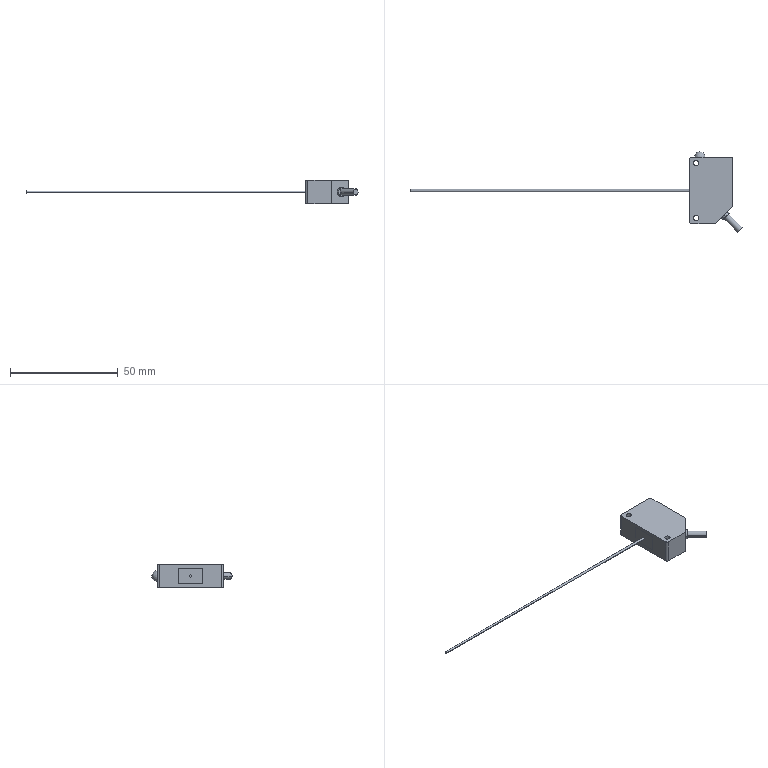Part | STEP file | ES201-R10MN (Huayifeng) | 1 solid | 26 faces | box 154.334 x 37.365 x 10.8 mm | volume 6448 mm3 | cylinder 13 | plane 11 | sphere 2 | commonest cylinder face diameters 2.5 x4 2 x3 1 x2 2.91 x2 4.315 x2
STEP:
#1=CARTESIAN_POINT('',(-140.,0.5,0.));
#2=VERTEX_POINT('',#1);
#3=CARTESIAN_POINT('',(-140.,-0.5,0.));
#4=VERTEX_POINT('',#3);
#5=CARTESIAN_POINT('',(-140.,0.,0.));
#6=DIRECTION('',(1.,0.,0.));
#7=DIRECTION('',(0.,-1.,0.));
#8=AXIS2_PLACEMENT_3D('',#5,#6,#7);
#9=CIRCLE('',#8,0.5);
#10=EDGE_CURVE('',#2,#4,#9,.T.);
#11=ORIENTED_EDGE('',*,*,#10,.T.);
#12=CARTESIAN_POINT('',(-10.,-0.5,0.));
#13=VERTEX_POINT('',#12);
#14=CARTESIAN_POINT('',(-140.,-0.5,0.));
#15=DIRECTION('',(1.,0.,0.));
#16=VECTOR('',#15,1000.);
#17=LINE('',#14,#16);
#18=EDGE_CURVE('',#4,#13,#17,.T.);
#19=ORIENTED_EDGE('',*,*,#18,.T.);
#20=CARTESIAN_POINT('',(-10.,0.5,0.));
#21=VERTEX_POINT('',#20);
#22=CARTESIAN_POINT('',(-10.,0.,0.));
#23=DIRECTION('',(1.,0.,0.));
#24=DIRECTION('',(0.,1.,0.));
#25=AXIS2_PLACEMENT_3D('',#22,#23,#24);
#26=CIRCLE('',#25,0.5);
#27=EDGE_CURVE('',#21,#13,#26,.T.);
#28=ORIENTED_EDGE('',*,*,#27,.F.);
#29=CARTESIAN_POINT('',(-140.,0.5,0.));
#30=DIRECTION('',(1.,0.,0.));
#31=VECTOR('',#30,1000.);
#32=LINE('',#29,#31);
#33=EDGE_CURVE('',#2,#21,#32,.T.);
#34=ORIENTED_EDGE('',*,*,#33,.F.);
#35=EDGE_LOOP('',(#11,#19,#28,#34));
#36=FACE_OUTER_BOUND('',#35,.T.);
#37=CARTESIAN_POINT('',(-140.,0.,0.));
#38=DIRECTION('',(1.,0.,0.));
#39=DIRECTION('',(0.,1.,0.));
#40=AXIS2_PLACEMENT_3D('',#37,#38,#39);
#41=CYLINDRICAL_SURFACE('',#40,0.5);
#42=ADVANCED_FACE('',(#36),#41,.T.);
#43=CARTESIAN_POINT('',(12.277,-19.365,0.));
#44=VERTEX_POINT('',#43);
#45=CARTESIAN_POINT('',(14.334,-17.308,0.));
#46=VERTEX_POINT('',#45);
#47=CARTESIAN_POINT('',(13.306,-18.336,0.));
#48=DIRECTION('',(-0.7071,0.7071,0.));
#49=DIRECTION('',(0.7071,0.7071,0.));
#50=AXIS2_PLACEMENT_3D('',#47,#48,#49);
#51=CIRCLE('',#50,1.455);
#52=EDGE_CURVE('',#44,#46,#51,.T.);
#53=ORIENTED_EDGE('',*,*,#52,.T.);
#54=CARTESIAN_POINT('',(7.97,-10.944,0.));
#55=VERTEX_POINT('',#54);
#56=CARTESIAN_POINT('',(14.334,-17.308,0.));
#57=DIRECTION('',(-0.7071,0.7071,0.));
#58=VECTOR('',#57,1000.);
#59=LINE('',#56,#58);
#60=EDGE_CURVE('',#46,#55,#59,.T.);
#61=ORIENTED_EDGE('',*,*,#60,.T.);
#62=CARTESIAN_POINT('',(5.913,-13.001,0.));
#63=VERTEX_POINT('',#62);
#64=CARTESIAN_POINT('',(6.942,-11.972,0.));
#65=DIRECTION('',(-0.7071,0.7071,0.));
#66=DIRECTION('',(0.7071,0.7071,0.));
#67=AXIS2_PLACEMENT_3D('',#64,#65,#66);
#68=CIRCLE('',#67,1.455);
#69=EDGE_CURVE('',#63,#55,#68,.T.);
#70=ORIENTED_EDGE('',*,*,#69,.F.);
#71=CARTESIAN_POINT('',(12.277,-19.365,0.));
#72=DIRECTION('',(-0.7071,0.7071,0.));
#73=VECTOR('',#72,1000.);
#74=LINE('',#71,#73);
#75=EDGE_CURVE('',#44,#63,#74,.T.);
#76=ORIENTED_EDGE('',*,*,#75,.F.);
#77=EDGE_LOOP('',(#53,#61,#70,#76));
#78=FACE_OUTER_BOUND('',#77,.T.);
#79=CARTESIAN_POINT('',(13.306,-18.336,0.));
#80=DIRECTION('',(-0.7071,0.7071,0.));
#81=DIRECTION('',(-0.7071,-0.7071,0.));
#82=AXIS2_PLACEMENT_3D('',#79,#80,#81);
#83=CYLINDRICAL_SURFACE('',#82,1.455);
#84=ADVANCED_FACE('',(#78),#83,.T.);
#85=CARTESIAN_POINT('',(5.416,-13.498,0.));
#86=VERTEX_POINT('',#85);
#87=CARTESIAN_POINT('',(8.467,-10.447,0.));
#88=VERTEX_POINT('',#87);
#89=CARTESIAN_POINT('',(6.942,-11.972,0.));
#90=DIRECTION('',(-0.7071,0.7071,0.));
#91=DIRECTION('',(0.7071,0.7071,0.));
#92=AXIS2_PLACEMENT_3D('',#89,#90,#91);
#93=CIRCLE('',#92,2.158);
#94=EDGE_CURVE('',#86,#88,#93,.T.);
#95=ORIENTED_EDGE('',*,*,#94,.T.);
#96=CARTESIAN_POINT('',(7.76,-9.74,0.));
#97=VERTEX_POINT('',#96);
#98=CARTESIAN_POINT('',(8.467,-10.447,0.));
#99=DIRECTION('',(-0.7071,0.7071,0.));
#100=VECTOR('',#99,1000.);
#101=LINE('',#98,#100);
#102=EDGE_CURVE('',#88,#97,#101,.T.);
#103=ORIENTED_EDGE('',*,*,#102,.T.);
#104=CARTESIAN_POINT('',(4.709,-12.791,0.));
#105=VERTEX_POINT('',#104);
#106=CARTESIAN_POINT('',(6.235,-11.265,0.));
#107=DIRECTION('',(-0.7071,0.7071,0.));
#108=DIRECTION('',(0.7071,0.7071,0.));
#109=AXIS2_PLACEMENT_3D('',#106,#107,#108);
#110=CIRCLE('',#109,2.158);
#111=EDGE_CURVE('',#105,#97,#110,.T.);
#112=ORIENTED_EDGE('',*,*,#111,.F.);
#113=CARTESIAN_POINT('',(5.416,-13.498,0.));
#114=DIRECTION('',(-0.7071,0.7071,0.));
#115=VECTOR('',#114,1000.);
#116=LINE('',#113,#115);
#117=EDGE_CURVE('',#86,#105,#116,.T.);
#118=ORIENTED_EDGE('',*,*,#117,.F.);
#119=EDGE_LOOP('',(#95,#103,#112,#118));
#120=FACE_OUTER_BOUND('',#119,.T.);
#121=CARTESIAN_POINT('',(6.942,-11.972,0.));
#122=DIRECTION('',(-0.7071,0.7071,0.));
#123=DIRECTION('',(-0.7071,-0.7071,0.));
#124=AXIS2_PLACEMENT_3D('',#121,#122,#123);
#125=CYLINDRICAL_SURFACE('',#124,2.158);
#126=ADVANCED_FACE('',(#120),#125,.T.);
#127=CARTESIAN_POINT('',(-5.75,-12.7,5.4));
#128=VERTEX_POINT('',#127);
#129=CARTESIAN_POINT('',(-8.25,-12.7,5.4));
#130=VERTEX_POINT('',#129);
#131=CARTESIAN_POINT('',(-7.,-12.7,5.4));
#132=DIRECTION('',(0.,0.,1.));
#133=DIRECTION('',(1.,0.,0.));
#134=AXIS2_PLACEMENT_3D('',#131,#132,#133);
#135=CIRCLE('',#134,1.25);
#136=EDGE_CURVE('',#128,#130,#135,.T.);
#137=ORIENTED_EDGE('',*,*,#136,.T.);
#138=CARTESIAN_POINT('',(-8.25,-12.7,-5.4));
#139=VERTEX_POINT('',#138);
#140=CARTESIAN_POINT('',(-8.25,-12.7,-5.4));
#141=DIRECTION('',(0.,0.,-1.));
#142=VECTOR('',#141,1000.);
#143=LINE('',#140,#142);
#144=EDGE_CURVE('',#130,#139,#143,.T.);
#145=ORIENTED_EDGE('',*,*,#144,.T.);
#146=CARTESIAN_POINT('',(-5.75,-12.7,-5.4));
#147=VERTEX_POINT('',#146);
#148=CARTESIAN_POINT('',(-7.,-12.7,-5.4));
#149=DIRECTION('',(0.,0.,1.));
#150=DIRECTION('',(1.,0.,0.));
#151=AXIS2_PLACEMENT_3D('',#148,#149,#150);
#152=CIRCLE('',#151,1.25);
#153=EDGE_CURVE('',#147,#139,#152,.T.);
#154=ORIENTED_EDGE('',*,*,#153,.F.);
#155=CARTESIAN_POINT('',(-5.75,-12.7,-5.4));
#156=DIRECTION('',(0.,0.,-1.));
#157=VECTOR('',#156,1000.);
#158=LINE('',#155,#157);
#159=EDGE_CURVE('',#128,#147,#158,.T.);
#160=ORIENTED_EDGE('',*,*,#159,.F.);
#161=EDGE_LOOP('',(#137,#145,#154,#160));
#162=FACE_OUTER_BOUND('',#161,.T.);
#163=CARTESIAN_POINT('',(-7.,-12.7,-5.4));
#164=DIRECTION('',(0.,0.,-1.));
#165=DIRECTION('',(1.,0.,0.));
#166=AXIS2_PLACEMENT_3D('',#163,#164,#165);
#167=CYLINDRICAL_SURFACE('',#166,1.25);
#168=ADVANCED_FACE('',(#162),#167,.F.);
#169=CARTESIAN_POINT('',(-7.176,13.938,0.));
#170=VERTEX_POINT('',#169);
#171=CARTESIAN_POINT('',(-5.806,13.069,-0.001365));
#172=VERTEX_POINT('',#171);
#173=CARTESIAN_POINT('',(-7.176,13.938,0.));
#174=CARTESIAN_POINT('',(-7.176,13.938,0.1523));
#175=CARTESIAN_POINT('',(-7.16,13.94,0.3021));
#176=CARTESIAN_POINT('',(-7.096,13.947,0.5968));
#177=CARTESIAN_POINT('',(-7.047,13.951,0.7424));
#178=CARTESIAN_POINT('',(-6.91,13.949,1.012));
#179=CARTESIAN_POINT('',(-6.821,13.943,1.139));
#180=CARTESIAN_POINT('',(-6.652,13.902,1.289));
#181=CARTESIAN_POINT('',(-6.592,13.884,1.331));
#182=CARTESIAN_POINT('',(-6.461,13.83,1.392));
#183=CARTESIAN_POINT('',(-6.393,13.795,1.408));
#184=CARTESIAN_POINT('',(-6.265,13.714,1.408));
#185=CARTESIAN_POINT('',(-6.205,13.667,1.391));
#186=CARTESIAN_POINT('',(-6.102,13.572,1.33));
#187=CARTESIAN_POINT('',(-6.059,13.525,1.287));
#188=CARTESIAN_POINT('',(-5.952,13.391,1.137));
#189=CARTESIAN_POINT('',(-5.908,13.313,1.011));
#190=CARTESIAN_POINT('',(-5.848,13.19,0.739));
#191=CARTESIAN_POINT('',(-5.831,13.145,0.5964));
#192=CARTESIAN_POINT('',(-5.81,13.084,0.3011));
#193=CARTESIAN_POINT('',(-5.806,13.069,0.1493));
#194=CARTESIAN_POINT('',(-5.806,13.069,-0.001365));
#195=B_SPLINE_CURVE_WITH_KNOTS('',3,(#173,#174,#175,#176,#177,#178,#179,#180,#181,#182,#183,#184,#185,#186,#187,#188,#189,#190,#191,#192,#193,#194),.UNSPECIFIED.,.F.,.F.,(4,2,2,2,2,2,2,2,2,2,4),(0.,0.0004516,0.0009031,0.001355,0.00158,0.001806,0.002032,0.002258,0.002709,0.003161,0.003613),.UNSPECIFIED.);
#196=EDGE_CURVE('',#170,#172,#195,.T.);
#197=ORIENTED_EDGE('',*,*,#196,.T.);
#198=CARTESIAN_POINT('',(-5.806,13.069,-0.001365));
#199=CARTESIAN_POINT('',(-5.806,13.069,-0.152));
#200=CARTESIAN_POINT('',(-5.81,13.084,-0.3044));
#201=CARTESIAN_POINT('',(-5.832,13.145,-0.5986));
#202=CARTESIAN_POINT('',(-5.848,13.191,-0.7422));
#203=CARTESIAN_POINT('',(-5.894,13.284,-0.9455));
#204=CARTESIAN_POINT('',(-5.913,13.318,-1.01));
#205=CARTESIAN_POINT('',(-5.96,13.395,-1.132));
#206=CARTESIAN_POINT('',(-5.989,13.437,-1.19));
#207=CARTESIAN_POINT('',(-6.06,13.526,-1.289));
#208=CARTESIAN_POINT('',(-6.104,13.574,-1.332));
#209=CARTESIAN_POINT('',(-6.207,13.669,-1.391));
#210=CARTESIAN_POINT('',(-6.267,13.715,-1.408));
#211=CARTESIAN_POINT('',(-6.395,13.797,-1.408));
#212=CARTESIAN_POINT('',(-6.463,13.831,-1.391));
#213=CARTESIAN_POINT('',(-6.593,13.884,-1.33));
#214=CARTESIAN_POINT('',(-6.654,13.903,-1.288));
#215=CARTESIAN_POINT('',(-6.822,13.943,-1.137));
#216=CARTESIAN_POINT('',(-6.911,13.949,-1.011));
#217=CARTESIAN_POINT('',(-7.047,13.951,-0.7418));
#218=CARTESIAN_POINT('',(-7.096,13.947,-0.5968));
#219=CARTESIAN_POINT('',(-7.16,13.94,-0.3018));
#220=CARTESIAN_POINT('',(-7.176,13.938,-0.1523));
#221=CARTESIAN_POINT('',(-7.176,13.938,0.));
#222=B_SPLINE_CURVE_WITH_KNOTS('',3,(#198,#199,#200,#201,#202,#203,#204,#205,#206,#207,#208,#209,#210,#211,#212,#213,#214,#215,#216,#217,#218,#219,#220,#221),.UNSPECIFIED.,.F.,.F.,(4,2,2,2,2,2,2,2,2,2,2,4),(0.003613,0.004064,0.004516,0.004741,0.004967,0.005193,0.005419,0.005645,0.00587,0.006322,0.006773,0.007225),.UNSPECIFIED.);
#223=EDGE_CURVE('',#172,#170,#222,.T.);
#224=ORIENTED_EDGE('',*,*,#223,.T.);
#225=EDGE_LOOP('',(#197,#224));
#226=FACE_BOUND('',#225,.T.);
#227=CARTESIAN_POINT('',(-5.75,12.7,5.4));
#228=VERTEX_POINT('',#227);
#229=CARTESIAN_POINT('',(-8.25,12.7,5.4));
#230=VERTEX_POINT('',#229);
#231=CARTESIAN_POINT('',(-7.,12.7,5.4));
#232=DIRECTION('',(0.,0.,1.));
#233=DIRECTION('',(1.,0.,0.));
#234=AXIS2_PLACEMENT_3D('',#231,#232,#233);
#235=CIRCLE('',#234,1.25);
#236=EDGE_CURVE('',#228,#230,#235,.T.);
#237=ORIENTED_EDGE('',*,*,#236,.T.);
#238=CARTESIAN_POINT('',(-8.25,12.7,-5.4));
#239=VERTEX_POINT('',#238);
#240=CARTESIAN_POINT('',(-8.25,12.7,-5.4));
#241=DIRECTION('',(0.,0.,-1.));
#242=VECTOR('',#241,1000.);
#243=LINE('',#240,#242);
#244=EDGE_CURVE('',#230,#239,#243,.T.);
#245=ORIENTED_EDGE('',*,*,#244,.T.);
#246=CARTESIAN_POINT('',(-5.75,12.7,-5.4));
#247=VERTEX_POINT('',#246);
#248=CARTESIAN_POINT('',(-7.,12.7,-5.4));
#249=DIRECTION('',(0.,0.,1.));
#250=DIRECTION('',(1.,0.,0.));
#251=AXIS2_PLACEMENT_3D('',#248,#249,#250);
#252=CIRCLE('',#251,1.25);
#253=EDGE_CURVE('',#247,#239,#252,.T.);
#254=ORIENTED_EDGE('',*,*,#253,.F.);
#255=CARTESIAN_POINT('',(-5.75,12.7,-5.4));
#256=DIRECTION('',(0.,0.,-1.));
#257=VECTOR('',#256,1000.);
#258=LINE('',#255,#257);
#259=EDGE_CURVE('',#228,#247,#258,.T.);
#260=ORIENTED_EDGE('',*,*,#259,.F.);
#261=EDGE_LOOP('',(#237,#245,#254,#260));
#262=FACE_OUTER_BOUND('',#261,.T.);
#263=CARTESIAN_POINT('',(-7.,12.7,-5.4));
#264=DIRECTION('',(0.,0.,-1.));
#265=DIRECTION('',(1.,0.,0.));
#266=AXIS2_PLACEMENT_3D('',#263,#264,#265);
#267=CYLINDRICAL_SURFACE('',#266,1.25);
#268=ADVANCED_FACE('',(#226,#262),#267,.F.);
#269=CARTESIAN_POINT('',(-10.,5.6,-3.7));
#270=VERTEX_POINT('',#269);
#271=CARTESIAN_POINT('',(-10.,5.6,3.7));
#272=VERTEX_POINT('',#271);
#273=CARTESIAN_POINT('',(-10.,5.6,-5.4));
#274=DIRECTION('',(0.,0.,1.));
#275=VECTOR('',#274,1000.);
#276=LINE('',#273,#275);
#277=EDGE_CURVE('',#270,#272,#276,.T.);
#278=ORIENTED_EDGE('',*,*,#277,.F.);
#279=CARTESIAN_POINT('',(-10.,-5.6,-3.7));
#280=VERTEX_POINT('',#279);
#281=CARTESIAN_POINT('',(-10.,15.5,-3.7));
#282=DIRECTION('',(0.,1.,0.));
#283=VECTOR('',#282,1000.);
#284=LINE('',#281,#283);
#285=EDGE_CURVE('',#280,#270,#284,.T.);
#286=ORIENTED_EDGE('',*,*,#285,.F.);
#287=CARTESIAN_POINT('',(-10.,-5.6,3.7));
#288=VERTEX_POINT('',#287);
#289=CARTESIAN_POINT('',(-10.,-5.6,-5.4));
#290=DIRECTION('',(0.,0.,-1.));
#291=VECTOR('',#290,1000.);
#292=LINE('',#289,#291);
#293=EDGE_CURVE('',#288,#280,#292,.T.);
#294=ORIENTED_EDGE('',*,*,#293,.F.);
#295=CARTESIAN_POINT('',(-10.,15.5,3.7));
#296=DIRECTION('',(0.,-1.,0.));
#297=VECTOR('',#296,1000.);
#298=LINE('',#295,#297);
#299=EDGE_CURVE('',#272,#288,#298,.T.);
#300=ORIENTED_EDGE('',*,*,#299,.F.);
#301=EDGE_LOOP('',(#278,#286,#294,#300));
#302=FACE_OUTER_BOUND('',#301,.T.);
#303=ORIENTED_EDGE('',*,*,#27,.T.);
#304=CARTESIAN_POINT('',(-10.,0.,0.));
#305=DIRECTION('',(1.,0.,0.));
#306=DIRECTION('',(0.,1.,0.));
#307=AXIS2_PLACEMENT_3D('',#304,#305,#306);
#308=CIRCLE('',#307,0.5);
#309=EDGE_CURVE('',#13,#21,#308,.T.);
#310=ORIENTED_EDGE('',*,*,#309,.T.);
#311=EDGE_LOOP('',(#303,#310));
#312=FACE_BOUND('',#311,.T.);
#313=CARTESIAN_POINT('',(-10.,15.5,-5.4));
#314=DIRECTION('',(1.,0.,0.));
#315=DIRECTION('',(0.,1.,0.));
#316=AXIS2_PLACEMENT_3D('',#313,#314,#315);
#317=PLANE('',#316);
#318=ADVANCED_FACE('',(#302,#312),#317,.F.);
#319=CARTESIAN_POINT('',(-10.,14.5,5.4));
#320=VERTEX_POINT('',#319);
#321=CARTESIAN_POINT('',(-10.,-14.5,5.4));
#322=VERTEX_POINT('',#321);
#323=CARTESIAN_POINT('',(-10.,15.5,5.4));
#324=DIRECTION('',(0.,-1.,0.));
#325=VECTOR('',#324,1000.);
#326=LINE('',#323,#325);
#327=EDGE_CURVE('',#320,#322,#326,.T.);
#328=ORIENTED_EDGE('',*,*,#327,.F.);
#329=CARTESIAN_POINT('',(-10.,14.5,-5.4));
#330=VERTEX_POINT('',#329);
#331=CARTESIAN_POINT('',(-10.,14.5,-5.4));
#332=DIRECTION('',(0.,0.,1.));
#333=VECTOR('',#332,1000.);
#334=LINE('',#331,#333);
#335=EDGE_CURVE('',#330,#320,#334,.T.);
#336=ORIENTED_EDGE('',*,*,#335,.F.);
#337=CARTESIAN_POINT('',(-10.,-14.5,-5.4));
#338=VERTEX_POINT('',#337);
#339=CARTESIAN_POINT('',(-10.,15.5,-5.4));
#340=DIRECTION('',(0.,-1.,0.));
#341=VECTOR('',#340,1000.);
#342=LINE('',#339,#341);
#343=EDGE_CURVE('',#330,#338,#342,.T.);
#344=ORIENTED_EDGE('',*,*,#343,.T.);
#345=CARTESIAN_POINT('',(-10.,-14.5,-5.4));
#346=DIRECTION('',(0.,0.,-1.));
#347=VECTOR('',#346,1000.);
#348=LINE('',#345,#347);
#349=EDGE_CURVE('',#322,#338,#348,.T.);
#350=ORIENTED_EDGE('',*,*,#349,.F.);
#351=EDGE_LOOP('',(#328,#336,#344,#350));
#352=FACE_OUTER_BOUND('',#351,.T.);
#353=ORIENTED_EDGE('',*,*,#299,.T.);
#354=ORIENTED_EDGE('',*,*,#293,.T.);
#355=ORIENTED_EDGE('',*,*,#285,.T.);
#356=ORIENTED_EDGE('',*,*,#277,.T.);
#357=EDGE_LOOP('',(#353,#354,#355,#356));
#358=FACE_BOUND('',#357,.T.);
#359=CARTESIAN_POINT('',(-10.,15.5,-5.4));
#360=DIRECTION('',(1.,0.,0.));
#361=DIRECTION('',(0.,1.,0.));
#362=AXIS2_PLACEMENT_3D('',#359,#360,#361);
#363=PLANE('',#362);
#364=ADVANCED_FACE('',(#352,#358),#363,.F.);
#365=ORIENTED_EDGE('',*,*,#94,.F.);
#366=CARTESIAN_POINT('',(6.942,-11.972,0.));
#367=DIRECTION('',(-0.7071,0.7071,0.));
#368=DIRECTION('',(0.7071,0.7071,0.));
#369=AXIS2_PLACEMENT_3D('',#366,#367,#368);
#370=CIRCLE('',#369,2.158);
#371=EDGE_CURVE('',#88,#86,#370,.T.);
#372=ORIENTED_EDGE('',*,*,#371,.F.);
#373=EDGE_LOOP('',(#365,#372));
#374=FACE_OUTER_BOUND('',#373,.T.);
#375=ORIENTED_EDGE('',*,*,#69,.T.);
#376=CARTESIAN_POINT('',(6.942,-11.972,0.));
#377=DIRECTION('',(-0.7071,0.7071,0.));
#378=DIRECTION('',(0.7071,0.7071,0.));
#379=AXIS2_PLACEMENT_3D('',#376,#377,#378);
#380=CIRCLE('',#379,1.455);
#381=EDGE_CURVE('',#55,#63,#380,.T.);
#382=ORIENTED_EDGE('',*,*,#381,.T.);
#383=EDGE_LOOP('',(#375,#382));
#384=FACE_BOUND('',#383,.T.);
#385=CARTESIAN_POINT('',(6.942,-11.972,0.));
#386=DIRECTION('',(0.7071,-0.7071,0.));
#387=DIRECTION('',(0.7071,0.7071,0.));
#388=AXIS2_PLACEMENT_3D('',#385,#386,#387);
#389=PLANE('',#388);
#390=ADVANCED_FACE('',(#374,#384),#389,.T.);
#391=CARTESIAN_POINT('',(2.,-15.5,-5.4));
#392=VERTEX_POINT('',#391);
#393=CARTESIAN_POINT('',(10.,-7.5,-5.4));
#394=VERTEX_POINT('',#393);
#395=CARTESIAN_POINT('',(6.,-11.5,-5.4));
#396=DIRECTION('',(0.7071,0.7071,0.));
#397=VECTOR('',#396,1000.);
#398=LINE('',#395,#397);
#399=EDGE_CURVE('',#392,#394,#398,.T.);
#400=ORIENTED_EDGE('',*,*,#399,.T.);
#401=CARTESIAN_POINT('',(10.,-7.5,5.4));
#402=VERTEX_POINT('',#401);
#403=CARTESIAN_POINT('',(10.,-7.5,-5.4));
#404=DIRECTION('',(0.,0.,1.));
#405=VECTOR('',#404,1000.);
#406=LINE('',#403,#405);
#407=EDGE_CURVE('',#394,#402,#406,.T.);
#408=ORIENTED_EDGE('',*,*,#407,.T.);
#409=CARTESIAN_POINT('',(2.,-15.5,5.4));
#410=VERTEX_POINT('',#409);
#411=CARTESIAN_POINT('',(10.,-7.5,5.4));
#412=DIRECTION('',(-0.7071,-0.7071,0.));
#413=VECTOR('',#412,1000.);
#414=LINE('',#411,#413);
#415=EDGE_CURVE('',#402,#410,#414,.T.);
#416=ORIENTED_EDGE('',*,*,#415,.T.);
#417=CARTESIAN_POINT('',(2.,-15.5,-5.4));
#418=DIRECTION('',(0.,0.,-1.));
#419=VECTOR('',#418,1000.);
#420=LINE('',#417,#419);
#421=EDGE_CURVE('',#410,#392,#420,.T.);
#422=ORIENTED_EDGE('',*,*,#421,.T.);
#423=EDGE_LOOP('',(#400,#408,#416,#422));
#424=FACE_OUTER_BOUND('',#423,.T.);
#425=ORIENTED_EDGE('',*,*,#111,.T.);
#426=CARTESIAN_POINT('',(6.235,-11.265,0.));
#427=DIRECTION('',(-0.7071,0.7071,0.));
#428=DIRECTION('',(0.7071,0.7071,0.));
#429=AXIS2_PLACEMENT_3D('',#426,#427,#428);
#430=CIRCLE('',#429,2.158);
#431=EDGE_CURVE('',#97,#105,#430,.T.);
#432=ORIENTED_EDGE('',*,*,#431,.T.);
#433=EDGE_LOOP('',(#425,#432));
#434=FACE_BOUND('',#433,.T.);
#435=CARTESIAN_POINT('',(10.,-7.5,-5.4));
#436=DIRECTION('',(-0.7071,0.7071,0.));
#437=DIRECTION('',(-0.7071,-0.7071,0.));
#438=AXIS2_PLACEMENT_3D('',#435,#436,#437);
#439=PLANE('',#438);
#440=ADVANCED_FACE('',(#424,#434),#439,.F.);
#441=CARTESIAN_POINT('',(9.,15.5,5.4));
#442=VERTEX_POINT('',#441);
#443=CARTESIAN_POINT('',(-9.,15.5,5.4));
#444=VERTEX_POINT('',#443);
#445=CARTESIAN_POINT('',(-10.,15.5,5.4));
#446=DIRECTION('',(-1.,0.,0.));
#447=VECTOR('',#446,1000.);
#448=LINE('',#445,#447);
#449=EDGE_CURVE('',#442,#444,#448,.T.);
#450=ORIENTED_EDGE('',*,*,#449,.F.);
#451=CARTESIAN_POINT('',(9.,15.5,-5.4));
#452=VERTEX_POINT('',#451);
#453=CARTESIAN_POINT('',(9.,15.5,-5.4));
#454=DIRECTION('',(0.,0.,1.));
#455=VECTOR('',#454,1000.);
#456=LINE('',#453,#455);
#457=EDGE_CURVE('',#452,#442,#456,.T.);
#458=ORIENTED_EDGE('',*,*,#457,.F.);
#459=CARTESIAN_POINT('',(-9.,15.5,-5.4));
#460=VERTEX_POINT('',#459);
#461=CARTESIAN_POINT('',(-10.,15.5,-5.4));
#462=DIRECTION('',(-1.,0.,0.));
#463=VECTOR('',#462,1000.);
#464=LINE('',#461,#463);
#465=EDGE_CURVE('',#452,#460,#464,.T.);
#466=ORIENTED_EDGE('',*,*,#465,.T.);
#467=CARTESIAN_POINT('',(-9.,15.5,-5.4));
#468=DIRECTION('',(0.,0.,-1.));
#469=VECTOR('',#468,1000.);
#470=LINE('',#467,#469);
#471=EDGE_CURVE('',#444,#460,#470,.T.);
#472=ORIENTED_EDGE('',*,*,#471,.F.);
#473=EDGE_LOOP('',(#450,#458,#466,#472));
#474=FACE_OUTER_BOUND('',#473,.T.);
#475=CARTESIAN_POINT('',(-5.224,15.5,2.5));
#476=VERTEX_POINT('',#475);
#477=CARTESIAN_POINT('',(-5.224,15.5,-2.5));
#478=VERTEX_POINT('',#477);
#479=CARTESIAN_POINT('',(-5.224,15.5,0.));
#480=DIRECTION('',(0.,-1.,0.));
#481=DIRECTION('',(0.,0.,1.));
#482=AXIS2_PLACEMENT_3D('',#479,#480,#481);
#483=CIRCLE('',#482,2.5);
#484=EDGE_CURVE('',#476,#478,#483,.T.);
#485=ORIENTED_EDGE('',*,*,#484,.T.);
#486=CARTESIAN_POINT('',(-5.224,15.5,0.));
#487=DIRECTION('',(0.,-1.,0.));
#488=DIRECTION('',(0.,0.,1.));
#489=AXIS2_PLACEMENT_3D('',#486,#487,#488);
#490=CIRCLE('',#489,2.5);
#491=EDGE_CURVE('',#478,#476,#490,.T.);
#492=ORIENTED_EDGE('',*,*,#491,.T.);
#493=EDGE_LOOP('',(#485,#492));
#494=FACE_BOUND('',#493,.T.);
#495=CARTESIAN_POINT('',(-10.,15.5,-5.4));
#496=DIRECTION('',(0.,-1.,0.));
#497=DIRECTION('',(0.,0.,1.));
#498=AXIS2_PLACEMENT_3D('',#495,#496,#497);
#499=PLANE('',#498);
#500=ADVANCED_FACE('',(#474,#494),#499,.F.);
#501=ORIENTED_EDGE('',*,*,#244,.F.);
#502=CARTESIAN_POINT('',(-7.,12.7,5.4));
#503=DIRECTION('',(0.,0.,1.));
#504=DIRECTION('',(1.,0.,0.));
#505=AXIS2_PLACEMENT_3D('',#502,#503,#504);
#506=CIRCLE('',#505,1.25);
#507=EDGE_CURVE('',#230,#228,#506,.T.);
#508=ORIENTED_EDGE('',*,*,#507,.T.);
#509=ORIENTED_EDGE('',*,*,#259,.T.);
#510=CARTESIAN_POINT('',(-7.,12.7,-5.4));
#511=DIRECTION('',(0.,0.,1.));
#512=DIRECTION('',(1.,0.,0.));
#513=AXIS2_PLACEMENT_3D('',#510,#511,#512);
#514=CIRCLE('',#513,1.25);
#515=EDGE_CURVE('',#239,#247,#514,.T.);
#516=ORIENTED_EDGE('',*,*,#515,.F.);
#517=EDGE_LOOP('',(#501,#508,#509,#516));
#518=FACE_OUTER_BOUND('',#517,.T.);
#519=CARTESIAN_POINT('',(-7.,12.7,-5.4));
#520=DIRECTION('',(0.,0.,-1.));
#521=DIRECTION('',(1.,0.,0.));
#522=AXIS2_PLACEMENT_3D('',#519,#520,#521);
#523=CYLINDRICAL_SURFACE('',#522,1.25);
#524=ADVANCED_FACE('',(#518),#523,.F.);
#525=CARTESIAN_POINT('',(10.,14.5,5.4));
#526=VERTEX_POINT('',#525);
#527=CARTESIAN_POINT('',(10.,15.5,5.4));
#528=DIRECTION('',(0.,1.,0.));
#529=VECTOR('',#528,1000.);
#530=LINE('',#527,#529);
#531=EDGE_CURVE('',#402,#526,#530,.T.);
#532=ORIENTED_EDGE('',*,*,#531,.F.);
#533=ORIENTED_EDGE('',*,*,#407,.F.);
#534=CARTESIAN_POINT('',(10.,14.5,-5.4));
#535=VERTEX_POINT('',#534);
#536=CARTESIAN_POINT('',(10.,15.5,-5.4));
#537=DIRECTION('',(0.,1.,0.));
#538=VECTOR('',#537,1000.);
#539=LINE('',#536,#538);
#540=EDGE_CURVE('',#394,#535,#539,.T.);
#541=ORIENTED_EDGE('',*,*,#540,.T.);
#542=CARTESIAN_POINT('',(10.,14.5,-5.4));
#543=DIRECTION('',(0.,0.,-1.));
#544=VECTOR('',#543,1000.);
#545=LINE('',#542,#544);
#546=EDGE_CURVE('',#526,#535,#545,.T.);
#547=ORIENTED_EDGE('',*,*,#546,.F.);
#548=EDGE_LOOP('',(#532,#533,#541,#547));
#549=FACE_OUTER_BOUND('',#548,.T.);
#550=CARTESIAN_POINT('',(10.,15.5,-5.4));
#551=DIRECTION('',(-1.,0.,0.));
#552=DIRECTION('',(0.,-1.,0.));
#553=AXIS2_PLACEMENT_3D('',#550,#551,#552);
#554=PLANE('',#553);
#555=ADVANCED_FACE('',(#549),#554,.F.);
#556=CARTESIAN_POINT('',(-9.,-15.5,-5.4));
#557=VERTEX_POINT('',#556);
#558=CARTESIAN_POINT('',(-10.,-15.5,-5.4));
#559=DIRECTION('',(1.,0.,0.));
#560=VECTOR('',#559,1000.);
#561=LINE('',#558,#560);
#562=EDGE_CURVE('',#557,#392,#561,.T.);
#563=ORIENTED_EDGE('',*,*,#562,.T.);
#564=ORIENTED_EDGE('',*,*,#421,.F.);
#565=CARTESIAN_POINT('',(-9.,-15.5,5.4));
#566=VERTEX_POINT('',#565);
#567=CARTESIAN_POINT('',(-10.,-15.5,5.4));
#568=DIRECTION('',(1.,0.,0.));
#569=VECTOR('',#568,1000.);
#570=LINE('',#567,#569);
#571=EDGE_CURVE('',#566,#410,#570,.T.);
#572=ORIENTED_EDGE('',*,*,#571,.F.);
#573=CARTESIAN_POINT('',(-9.,-15.5,-5.4));
#574=DIRECTION('',(0.,0.,1.));
#575=VECTOR('',#574,1000.);
#576=LINE('',#573,#575);
#577=EDGE_CURVE('',#557,#566,#576,.T.);
#578=ORIENTED_EDGE('',*,*,#577,.F.);
#579=EDGE_LOOP('',(#563,#564,#572,#578));
#580=FACE_OUTER_BOUND('',#579,.T.);
#581=CARTESIAN_POINT('',(-10.,-15.5,-5.4));
#582=DIRECTION('',(0.,1.,0.));
#583=DIRECTION('',(0.,0.,-1.));
#584=AXIS2_PLACEMENT_3D('',#581,#582,#583);
#585=PLANE('',#584);
#586=ADVANCED_FACE('',(#580),#585,.F.);
#587=ORIENTED_EDGE('',*,*,#253,.T.);
#588=ORIENTED_EDGE('',*,*,#515,.T.);
#589=EDGE_LOOP('',(#587,#588));
#590=FACE_BOUND('',#589,.T.);
#591=ORIENTED_EDGE('',*,*,#153,.T.);
#592=CARTESIAN_POINT('',(-7.,-12.7,-5.4));
#593=DIRECTION('',(0.,0.,1.));
#594=DIRECTION('',(1.,0.,0.));
#595=AXIS2_PLACEMENT_3D('',#592,#593,#594);
#596=CIRCLE('',#595,1.25);
#597=EDGE_CURVE('',#139,#147,#596,.T.);
#598=ORIENTED_EDGE('',*,*,#597,.T.);
#599=EDGE_LOOP('',(#591,#598));
#600=FACE_BOUND('',#599,.T.);
#601=ORIENTED_EDGE('',*,*,#343,.F.);
#602=CARTESIAN_POINT('',(-9.,14.5,-5.4));
#603=DIRECTION('',(0.,0.,1.));
#604=DIRECTION('',(1.,0.,0.));
#605=AXIS2_PLACEMENT_3D('',#602,#603,#604);
#606=CIRCLE('',#605,1.);
#607=EDGE_CURVE('',#460,#330,#606,.T.);
#608=ORIENTED_EDGE('',*,*,#607,.F.);
#609=ORIENTED_EDGE('',*,*,#465,.F.);
#610=CARTESIAN_POINT('',(9.,14.5,-5.4));
#611=DIRECTION('',(0.,0.,1.));
#612=DIRECTION('',(1.,0.,0.));
#613=AXIS2_PLACEMENT_3D('',#610,#611,#612);
#614=CIRCLE('',#613,1.);
#615=EDGE_CURVE('',#535,#452,#614,.T.);
#616=ORIENTED_EDGE('',*,*,#615,.F.);
#617=ORIENTED_EDGE('',*,*,#540,.F.);
#618=ORIENTED_EDGE('',*,*,#399,.F.);
#619=ORIENTED_EDGE('',*,*,#562,.F.);
#620=CARTESIAN_POINT('',(-9.,-14.5,-5.4));
#621=DIRECTION('',(0.,0.,1.));
#622=DIRECTION('',(1.,0.,0.));
#623=AXIS2_PLACEMENT_3D('',#620,#621,#622);
#624=CIRCLE('',#623,1.);
#625=EDGE_CURVE('',#338,#557,#624,.T.);
#626=ORIENTED_EDGE('',*,*,#625,.F.);
#627=EDGE_LOOP('',(#601,#608,#609,#616,#617,#618,#619,#626));
#628=FACE_OUTER_BOUND('',#627,.T.);
#629=CARTESIAN_POINT('',(10.,-15.5,-5.4));
#630=DIRECTION('',(0.,0.,-1.));
#631=DIRECTION('',(1.,0.,0.));
#632=AXIS2_PLACEMENT_3D('',#629,#630,#631);
#633=PLANE('',#632);
#634=ADVANCED_FACE('',(#590,#600,#628),#633,.T.);
#635=ORIENTED_EDGE('',*,*,#236,.F.);
#636=ORIENTED_EDGE('',*,*,#507,.F.);
#637=EDGE_LOOP('',(#635,#636));
#638=FACE_BOUND('',#637,.T.);
#639=ORIENTED_EDGE('',*,*,#136,.F.);
#640=CARTESIAN_POINT('',(-7.,-12.7,5.4));
#641=DIRECTION('',(0.,0.,1.));
#642=DIRECTION('',(1.,0.,0.));
#643=AXIS2_PLACEMENT_3D('',#640,#641,#642);
#644=CIRCLE('',#643,1.25);
#645=EDGE_CURVE('',#130,#128,#644,.T.);
#646=ORIENTED_EDGE('',*,*,#645,.F.);
#647=EDGE_LOOP('',(#639,#646));
#648=FACE_BOUND('',#647,.T.);
#649=ORIENTED_EDGE('',*,*,#571,.T.);
#650=ORIENTED_EDGE('',*,*,#415,.F.);
#651=ORIENTED_EDGE('',*,*,#531,.T.);
#652=CARTESIAN_POINT('',(9.,14.5,5.4));
#653=DIRECTION('',(0.,0.,-1.));
#654=DIRECTION('',(1.,0.,0.));
#655=AXIS2_PLACEMENT_3D('',#652,#653,#654);
#656=CIRCLE('',#655,1.);
#657=EDGE_CURVE('',#442,#526,#656,.T.);
#658=ORIENTED_EDGE('',*,*,#657,.F.);
#659=ORIENTED_EDGE('',*,*,#449,.T.);
#660=CARTESIAN_POINT('',(-9.,14.5,5.4));
#661=DIRECTION('',(0.,0.,-1.));
#662=DIRECTION('',(1.,0.,0.));
#663=AXIS2_PLACEMENT_3D('',#660,#661,#662);
#664=CIRCLE('',#663,1.);
#665=EDGE_CURVE('',#320,#444,#664,.T.);
#666=ORIENTED_EDGE('',*,*,#665,.F.);
#667=ORIENTED_EDGE('',*,*,#327,.T.);
#668=CARTESIAN_POINT('',(-9.,-14.5,5.4));
#669=DIRECTION('',(0.,0.,-1.));
#670=DIRECTION('',(1.,0.,0.));
#671=AXIS2_PLACEMENT_3D('',#668,#669,#670);
#672=CIRCLE('',#671,1.);
#673=EDGE_CURVE('',#566,#322,#672,.T.);
#674=ORIENTED_EDGE('',*,*,#673,.F.);
#675=EDGE_LOOP('',(#649,#650,#651,#658,#659,#666,#667,#674));
#676=FACE_OUTER_BOUND('',#675,.T.);
#677=CARTESIAN_POINT('',(10.,-15.5,5.4));
#678=DIRECTION('',(0.,0.,-1.));
#679=DIRECTION('',(1.,0.,0.));
#680=AXIS2_PLACEMENT_3D('',#677,#678,#679);
#681=PLANE('',#680);
#682=ADVANCED_FACE('',(#638,#648,#676),#681,.F.);
#683=ORIENTED_EDGE('',*,*,#144,.F.);
#684=ORIENTED_EDGE('',*,*,#645,.T.);
#685=ORIENTED_EDGE('',*,*,#159,.T.);
#686=ORIENTED_EDGE('',*,*,#597,.F.);
#687=EDGE_LOOP('',(#683,#684,#685,#686));
#688=FACE_OUTER_BOUND('',#687,.T.);
#689=CARTESIAN_POINT('',(-7.,-12.7,-5.4));
#690=DIRECTION('',(0.,0.,-1.));
#691=DIRECTION('',(1.,0.,0.));
#692=AXIS2_PLACEMENT_3D('',#689,#690,#691);
#693=CYLINDRICAL_SURFACE('',#692,1.25);
#694=ADVANCED_FACE('',(#688),#693,.F.);
#695=ORIENTED_EDGE('',*,*,#196,.F.);
#696=ORIENTED_EDGE('',*,*,#223,.F.);
#697=EDGE_LOOP('',(#695,#696));
#698=FACE_OUTER_BOUND('',#697,.T.);
#699=CARTESIAN_POINT('',(-5.224,15.5,0.));
#700=DIRECTION('',(0.,-1.,0.));
#701=DIRECTION('',(0.,0.,-1.));
#702=AXIS2_PLACEMENT_3D('',#699,#700,#701);
#703=SPHERICAL_SURFACE('',#702,2.5);
#704=ADVANCED_FACE('',(#698),#703,.T.);
#705=ORIENTED_EDGE('',*,*,#484,.F.);
#706=ORIENTED_EDGE('',*,*,#491,.F.);
#707=EDGE_LOOP('',(#705,#706));
#708=FACE_OUTER_BOUND('',#707,.T.);
#709=CARTESIAN_POINT('',(-5.224,15.5,0.));
#710=DIRECTION('',(0.,-1.,0.));
#711=DIRECTION('',(0.,0.,-1.));
#712=AXIS2_PLACEMENT_3D('',#709,#710,#711);
#713=SPHERICAL_SURFACE('',#712,2.5);
#714=ADVANCED_FACE('',(#708),#713,.T.);
#715=ORIENTED_EDGE('',*,*,#102,.F.);
#716=ORIENTED_EDGE('',*,*,#371,.T.);
#717=ORIENTED_EDGE('',*,*,#117,.T.);
#718=ORIENTED_EDGE('',*,*,#431,.F.);
#719=EDGE_LOOP('',(#715,#716,#717,#718));
#720=FACE_OUTER_BOUND('',#719,.T.);
#721=CARTESIAN_POINT('',(6.942,-11.972,0.));
#722=DIRECTION('',(-0.7071,0.7071,0.));
#723=DIRECTION('',(-0.7071,-0.7071,0.));
#724=AXIS2_PLACEMENT_3D('',#721,#722,#723);
#725=CYLINDRICAL_SURFACE('',#724,2.158);
#726=ADVANCED_FACE('',(#720),#725,.T.);
#727=ORIENTED_EDGE('',*,*,#60,.F.);
#728=CARTESIAN_POINT('',(13.306,-18.336,0.));
#729=DIRECTION('',(-0.7071,0.7071,0.));
#730=DIRECTION('',(0.7071,0.7071,0.));
#731=AXIS2_PLACEMENT_3D('',#728,#729,#730);
#732=CIRCLE('',#731,1.455);
#733=EDGE_CURVE('',#46,#44,#732,.T.);
#734=ORIENTED_EDGE('',*,*,#733,.T.);
#735=ORIENTED_EDGE('',*,*,#75,.T.);
#736=ORIENTED_EDGE('',*,*,#381,.F.);
#737=EDGE_LOOP('',(#727,#734,#735,#736));
#738=FACE_OUTER_BOUND('',#737,.T.);
#739=CARTESIAN_POINT('',(13.306,-18.336,0.));
#740=DIRECTION('',(-0.7071,0.7071,0.));
#741=DIRECTION('',(-0.7071,-0.7071,0.));
#742=AXIS2_PLACEMENT_3D('',#739,#740,#741);
#743=CYLINDRICAL_SURFACE('',#742,1.455);
#744=ADVANCED_FACE('',(#738),#743,.T.);
#745=ORIENTED_EDGE('',*,*,#52,.F.);
#746=ORIENTED_EDGE('',*,*,#733,.F.);
#747=EDGE_LOOP('',(#745,#746));
#748=FACE_OUTER_BOUND('',#747,.T.);
#749=CARTESIAN_POINT('',(13.306,-18.336,0.));
#750=DIRECTION('',(0.7071,-0.7071,0.));
#751=DIRECTION('',(0.7071,0.7071,0.));
#752=AXIS2_PLACEMENT_3D('',#749,#750,#751);
#753=PLANE('',#752);
#754=ADVANCED_FACE('',(#748),#753,.T.);
#755=ORIENTED_EDGE('',*,*,#625,.T.);
#756=ORIENTED_EDGE('',*,*,#577,.T.);
#757=ORIENTED_EDGE('',*,*,#673,.T.);
#758=ORIENTED_EDGE('',*,*,#349,.T.);
#759=EDGE_LOOP('',(#755,#756,#757,#758));
#760=FACE_OUTER_BOUND('',#759,.T.);
#761=CARTESIAN_POINT('',(-9.,-14.5,-5.4));
#762=DIRECTION('',(0.,0.,1.));
#763=DIRECTION('',(-1.,0.,0.));
#764=AXIS2_PLACEMENT_3D('',#761,#762,#763);
#765=CYLINDRICAL_SURFACE('',#764,1.);
#766=ADVANCED_FACE('',(#760),#765,.T.);
#767=ORIENTED_EDGE('',*,*,#607,.T.);
#768=ORIENTED_EDGE('',*,*,#335,.T.);
#769=ORIENTED_EDGE('',*,*,#665,.T.);
#770=ORIENTED_EDGE('',*,*,#471,.T.);
#771=EDGE_LOOP('',(#767,#768,#769,#770));
#772=FACE_OUTER_BOUND('',#771,.T.);
#773=CARTESIAN_POINT('',(-9.,14.5,-5.4));
#774=DIRECTION('',(0.,0.,1.));
#775=DIRECTION('',(-1.,0.,0.));
#776=AXIS2_PLACEMENT_3D('',#773,#774,#775);
#777=CYLINDRICAL_SURFACE('',#776,1.);
#778=ADVANCED_FACE('',(#772),#777,.T.);
#779=ORIENTED_EDGE('',*,*,#615,.T.);
#780=ORIENTED_EDGE('',*,*,#457,.T.);
#781=ORIENTED_EDGE('',*,*,#657,.T.);
#782=ORIENTED_EDGE('',*,*,#546,.T.);
#783=EDGE_LOOP('',(#779,#780,#781,#782));
#784=FACE_OUTER_BOUND('',#783,.T.);
#785=CARTESIAN_POINT('',(9.,14.5,-5.4));
#786=DIRECTION('',(0.,0.,1.));
#787=DIRECTION('',(-1.,0.,0.));
#788=AXIS2_PLACEMENT_3D('',#785,#786,#787);
#789=CYLINDRICAL_SURFACE('',#788,1.);
#790=ADVANCED_FACE('',(#784),#789,.T.);
#791=ORIENTED_EDGE('',*,*,#18,.F.);
#792=CARTESIAN_POINT('',(-140.,0.,0.));
#793=DIRECTION('',(1.,0.,0.));
#794=DIRECTION('',(0.,-1.,0.));
#795=AXIS2_PLACEMENT_3D('',#792,#793,#794);
#796=CIRCLE('',#795,0.5);
#797=EDGE_CURVE('',#4,#2,#796,.T.);
#798=ORIENTED_EDGE('',*,*,#797,.T.);
#799=ORIENTED_EDGE('',*,*,#33,.T.);
#800=ORIENTED_EDGE('',*,*,#309,.F.);
#801=EDGE_LOOP('',(#791,#798,#799,#800));
#802=FACE_OUTER_BOUND('',#801,.T.);
#803=CARTESIAN_POINT('',(-140.,0.,0.));
#804=DIRECTION('',(1.,0.,0.));
#805=DIRECTION('',(0.,1.,0.));
#806=AXIS2_PLACEMENT_3D('',#803,#804,#805);
#807=CYLINDRICAL_SURFACE('',#806,0.5);
#808=ADVANCED_FACE('',(#802),#807,.T.);
#809=ORIENTED_EDGE('',*,*,#10,.F.);
#810=ORIENTED_EDGE('',*,*,#797,.F.);
#811=EDGE_LOOP('',(#809,#810));
#812=FACE_OUTER_BOUND('',#811,.T.);
#813=CARTESIAN_POINT('',(-140.,0.,0.));
#814=DIRECTION('',(-1.,0.,0.));
#815=DIRECTION('',(0.,-1.,0.));
#816=AXIS2_PLACEMENT_3D('',#813,#814,#815);
#817=PLANE('',#816);
#818=ADVANCED_FACE('',(#812),#817,.T.);
#819=CLOSED_SHELL('',(#42,#84,#126,#168,#268,#318,#364,#390,#440,#500,#524,#555,#586,#634,#682,#694,#704,#714,#726,#744,#754,#766,#778,#790,#808,#818));
#820=MANIFOLD_SOLID_BREP('',#819);
#821=CARTESIAN_POINT('',(0.,0.,0.));
#822=DIRECTION('',(0.,0.,1.));
#823=DIRECTION('',(1.,0.,0.));
#824=AXIS2_PLACEMENT_3D('',#821,#822,#823);
#825=(LENGTH_UNIT()NAMED_UNIT(*)SI_UNIT(.MILLI.,.METRE.));
#826=UNCERTAINTY_MEASURE_WITH_UNIT(LENGTH_MEASURE(0.00001),#825,'','');
#827=(NAMED_UNIT(*)PLANE_ANGLE_UNIT()SI_UNIT($,.RADIAN.));
#828=(NAMED_UNIT(*)SI_UNIT($,.STERADIAN.)SOLID_ANGLE_UNIT());
#829=(GEOMETRIC_REPRESENTATION_CONTEXT(3)GLOBAL_UNCERTAINTY_ASSIGNED_CONTEXT((#826))GLOBAL_UNIT_ASSIGNED_CONTEXT((#825,#827,#828))REPRESENTATION_CONTEXT('',''));
#830=ADVANCED_BREP_SHAPE_REPRESENTATION('',(#820,#824),#829);